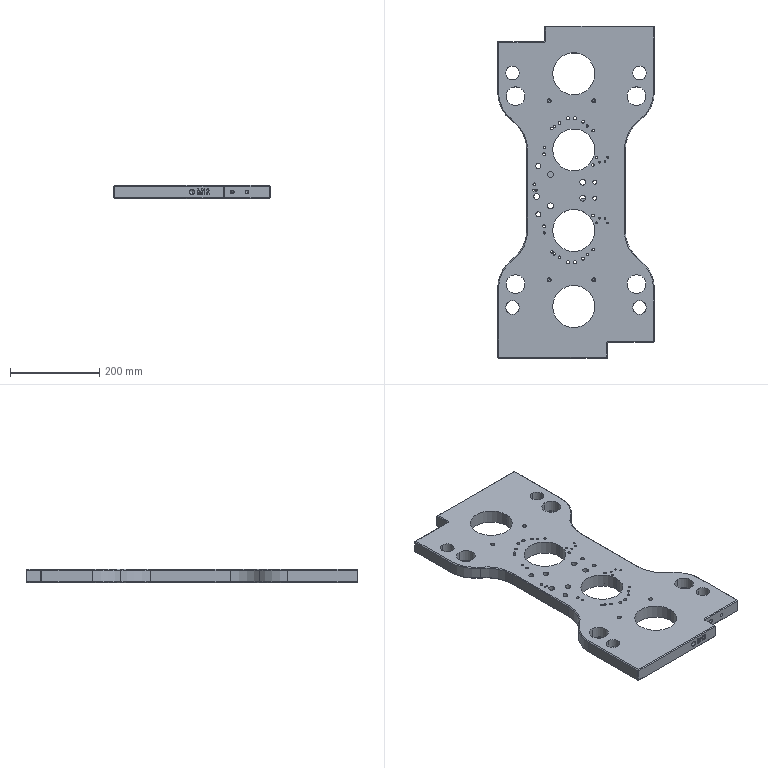Part | Creo | 1 solid | 682 faces | box 350 x 742 x 30 mm | volume 5147827 mm3 | cylinder 284 | plane 233 | other 91 | cone 74 | commonest cylinder face diameters 11 x45 8.5 x26 9 x22 7 x21 4 x20 6 x14